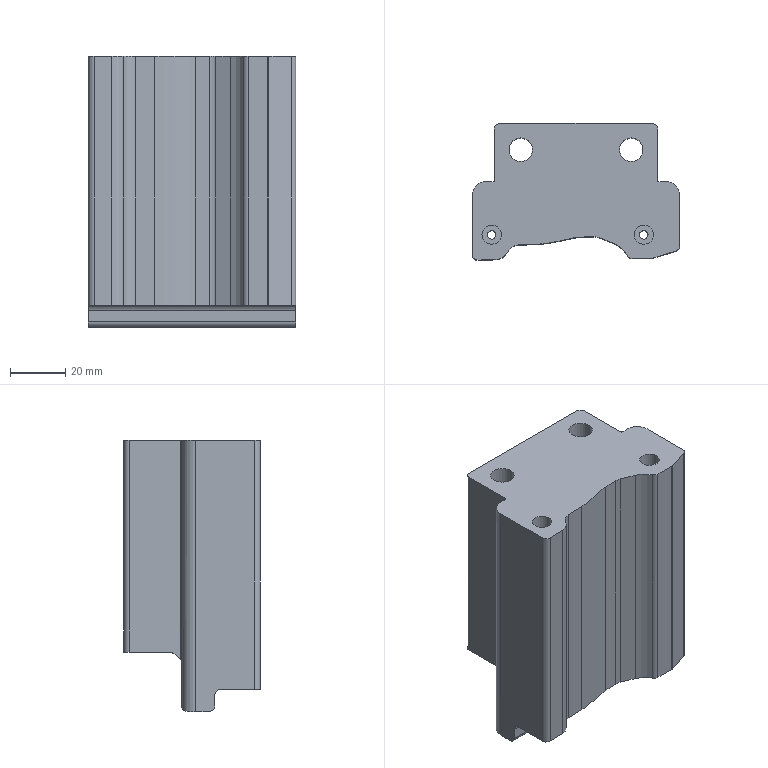Part | NX | features PU-7 2 | 1 solid | 48 faces | box 75 x 49.398 x 98 mm | volume 248578 mm3 | cylinder 22 | plane 19 | spline 7 | commonest cylinder face diameters 4 x9 10 x3 1 x2 3.101 x2 7 x2 8.506 x2